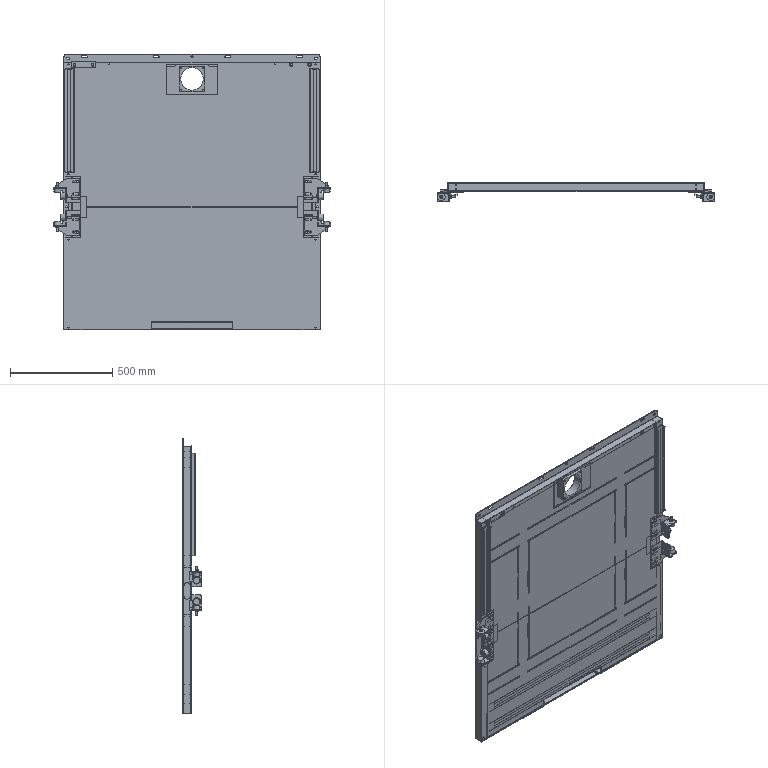Part | SolidWorks | features ReferencePattern 8, MirrorCompFeat 5 | 59 solids | 2152 faces | box 1354 x 89.5 x 1345 mm | volume 7454368 mm3 | plane 1446 | cylinder 586 | cone 120 | commonest cylinder face diameters 10 x112 0.4 x74 11 x61 3.4 x48 20 x39 9 x32